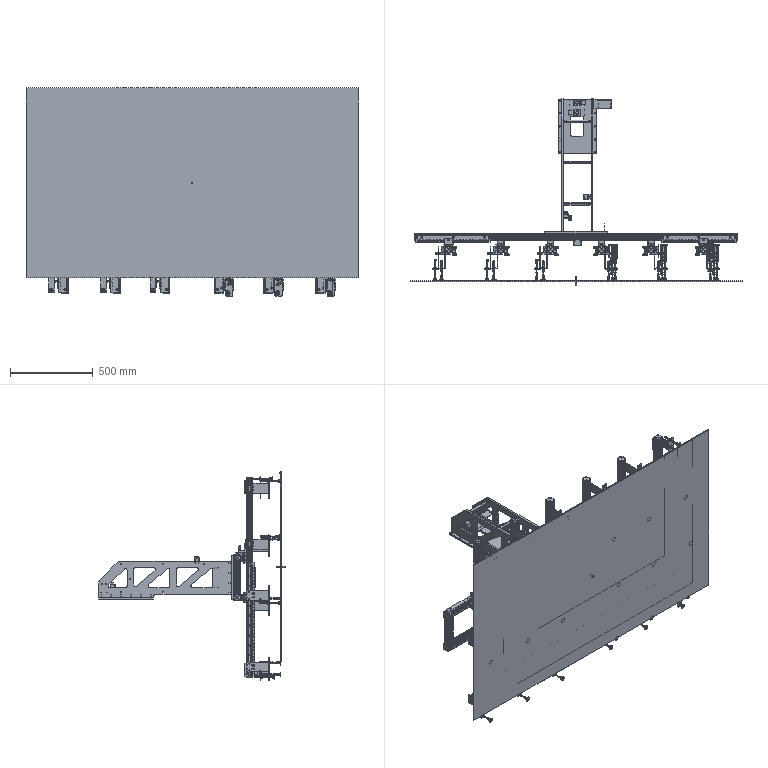Part | SolidWorks | features ReferencePattern 4, CompositeCurve 1, DerivedHolePattern 1 | 324 solids | 25513 faces | volume 31071679 mm3 | plane 11261 | cylinder 7985 | cone 4313 | spline 1954 | commonest cylinder face diameters 4.1 x484 4 x414 7 x365 6 x357 8 x352 10 x350